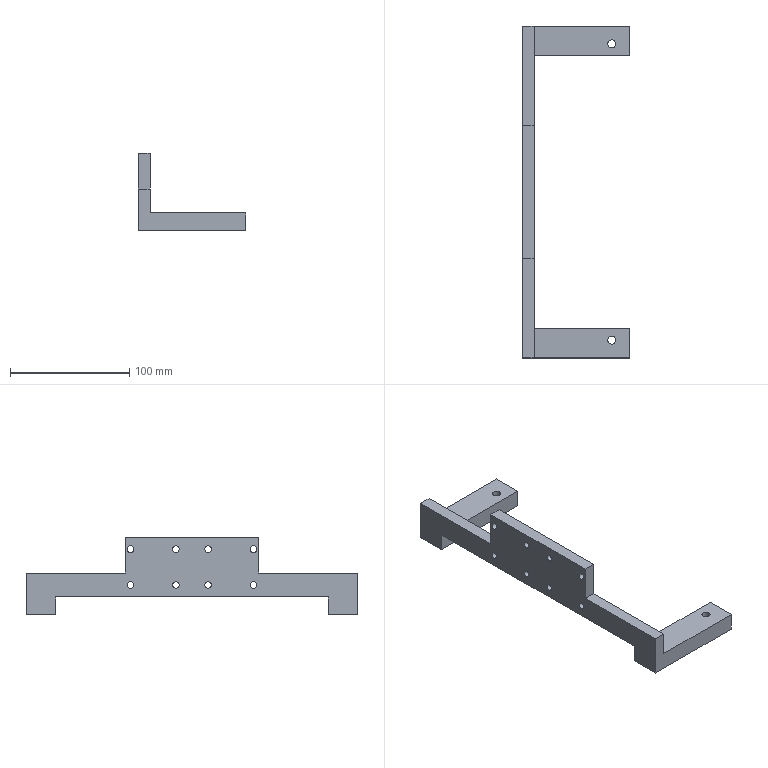Part | 1 solid | 38 faces | box 90 x 278 x 65 mm | volume 153710 mm3 | cylinder 20 | plane 18 | commonest cylinder face diameters 5.5 x16 6.8 x4
STEP:
#1=CARTESIAN_POINT('',(10.,148.5,17.25));
#2=VERTEX_POINT('',#1);
#3=CARTESIAN_POINT('',(10.,148.5,22.75));
#4=VERTEX_POINT('',#3);
#5=CARTESIAN_POINT('',(10.,148.5,20.));
#6=DIRECTION('',(-1.,0.,0.));
#7=DIRECTION('',(0.,0.,1.));
#8=AXIS2_PLACEMENT_3D('',#5,#6,#7);
#9=CIRCLE('',#8,2.75);
#10=EDGE_CURVE('',#2,#4,#9,.T.);
#11=ORIENTED_EDGE('',*,*,#10,.F.);
#12=CARTESIAN_POINT('',(0.,148.5,17.25));
#13=VERTEX_POINT('',#12);
#14=CARTESIAN_POINT('',(10.,148.5,17.25));
#15=DIRECTION('',(-1.,0.,0.));
#16=VECTOR('',#15,1000.);
#17=LINE('',#14,#16);
#18=EDGE_CURVE('',#2,#13,#17,.T.);
#19=ORIENTED_EDGE('',*,*,#18,.T.);
#20=CARTESIAN_POINT('',(0.,148.5,22.75));
#21=VERTEX_POINT('',#20);
#22=CARTESIAN_POINT('',(0.,148.5,20.));
#23=DIRECTION('',(-1.,0.,0.));
#24=DIRECTION('',(0.,0.,1.));
#25=AXIS2_PLACEMENT_3D('',#22,#23,#24);
#26=CIRCLE('',#25,2.75);
#27=EDGE_CURVE('',#13,#21,#26,.T.);
#28=ORIENTED_EDGE('',*,*,#27,.T.);
#29=CARTESIAN_POINT('',(10.,148.5,22.75));
#30=DIRECTION('',(-1.,0.,0.));
#31=VECTOR('',#30,1000.);
#32=LINE('',#29,#31);
#33=EDGE_CURVE('',#4,#21,#32,.T.);
#34=ORIENTED_EDGE('',*,*,#33,.F.);
#35=EDGE_LOOP('',(#11,#19,#28,#34));
#36=FACE_OUTER_BOUND('',#35,.T.);
#37=CARTESIAN_POINT('',(10.,148.5,20.));
#38=DIRECTION('',(-1.,0.,0.));
#39=DIRECTION('',(0.,0.,1.));
#40=AXIS2_PLACEMENT_3D('',#37,#38,#39);
#41=CYLINDRICAL_SURFACE('',#40,2.75);
#42=ADVANCED_FACE('',(#36),#41,.F.);
#43=CARTESIAN_POINT('',(10.,186.5,17.25));
#44=VERTEX_POINT('',#43);
#45=CARTESIAN_POINT('',(10.,186.5,22.75));
#46=VERTEX_POINT('',#45);
#47=CARTESIAN_POINT('',(10.,186.5,20.));
#48=DIRECTION('',(-1.,0.,0.));
#49=DIRECTION('',(0.,0.,1.));
#50=AXIS2_PLACEMENT_3D('',#47,#48,#49);
#51=CIRCLE('',#50,2.75);
#52=EDGE_CURVE('',#44,#46,#51,.T.);
#53=ORIENTED_EDGE('',*,*,#52,.F.);
#54=CARTESIAN_POINT('',(0.,186.5,17.25));
#55=VERTEX_POINT('',#54);
#56=CARTESIAN_POINT('',(10.,186.5,17.25));
#57=DIRECTION('',(-1.,0.,0.));
#58=VECTOR('',#57,1000.);
#59=LINE('',#56,#58);
#60=EDGE_CURVE('',#44,#55,#59,.T.);
#61=ORIENTED_EDGE('',*,*,#60,.T.);
#62=CARTESIAN_POINT('',(0.,186.5,22.75));
#63=VERTEX_POINT('',#62);
#64=CARTESIAN_POINT('',(0.,186.5,20.));
#65=DIRECTION('',(-1.,0.,0.));
#66=DIRECTION('',(0.,0.,1.));
#67=AXIS2_PLACEMENT_3D('',#64,#65,#66);
#68=CIRCLE('',#67,2.75);
#69=EDGE_CURVE('',#55,#63,#68,.T.);
#70=ORIENTED_EDGE('',*,*,#69,.T.);
#71=CARTESIAN_POINT('',(10.,186.5,22.75));
#72=DIRECTION('',(-1.,0.,0.));
#73=VECTOR('',#72,1000.);
#74=LINE('',#71,#73);
#75=EDGE_CURVE('',#46,#63,#74,.T.);
#76=ORIENTED_EDGE('',*,*,#75,.F.);
#77=EDGE_LOOP('',(#53,#61,#70,#76));
#78=FACE_OUTER_BOUND('',#77,.T.);
#79=CARTESIAN_POINT('',(10.,186.5,20.));
#80=DIRECTION('',(-1.,0.,0.));
#81=DIRECTION('',(0.,0.,1.));
#82=AXIS2_PLACEMENT_3D('',#79,#80,#81);
#83=CYLINDRICAL_SURFACE('',#82,2.75);
#84=ADVANCED_FACE('',(#78),#83,.F.);
#85=CARTESIAN_POINT('',(10.,148.5,47.25));
#86=VERTEX_POINT('',#85);
#87=CARTESIAN_POINT('',(10.,148.5,52.75));
#88=VERTEX_POINT('',#87);
#89=CARTESIAN_POINT('',(10.,148.5,50.));
#90=DIRECTION('',(-1.,0.,0.));
#91=DIRECTION('',(0.,0.,1.));
#92=AXIS2_PLACEMENT_3D('',#89,#90,#91);
#93=CIRCLE('',#92,2.75);
#94=EDGE_CURVE('',#86,#88,#93,.T.);
#95=ORIENTED_EDGE('',*,*,#94,.F.);
#96=CARTESIAN_POINT('',(0.,148.5,47.25));
#97=VERTEX_POINT('',#96);
#98=CARTESIAN_POINT('',(10.,148.5,47.25));
#99=DIRECTION('',(-1.,0.,0.));
#100=VECTOR('',#99,1000.);
#101=LINE('',#98,#100);
#102=EDGE_CURVE('',#86,#97,#101,.T.);
#103=ORIENTED_EDGE('',*,*,#102,.T.);
#104=CARTESIAN_POINT('',(0.,148.5,52.75));
#105=VERTEX_POINT('',#104);
#106=CARTESIAN_POINT('',(0.,148.5,50.));
#107=DIRECTION('',(-1.,0.,0.));
#108=DIRECTION('',(0.,0.,1.));
#109=AXIS2_PLACEMENT_3D('',#106,#107,#108);
#110=CIRCLE('',#109,2.75);
#111=EDGE_CURVE('',#97,#105,#110,.T.);
#112=ORIENTED_EDGE('',*,*,#111,.T.);
#113=CARTESIAN_POINT('',(10.,148.5,52.75));
#114=DIRECTION('',(-1.,0.,0.));
#115=VECTOR('',#114,1000.);
#116=LINE('',#113,#115);
#117=EDGE_CURVE('',#88,#105,#116,.T.);
#118=ORIENTED_EDGE('',*,*,#117,.F.);
#119=EDGE_LOOP('',(#95,#103,#112,#118));
#120=FACE_OUTER_BOUND('',#119,.T.);
#121=CARTESIAN_POINT('',(10.,148.5,50.));
#122=DIRECTION('',(-1.,0.,0.));
#123=DIRECTION('',(0.,0.,1.));
#124=AXIS2_PLACEMENT_3D('',#121,#122,#123);
#125=CYLINDRICAL_SURFACE('',#124,2.75);
#126=ADVANCED_FACE('',(#120),#125,.F.);
#127=CARTESIAN_POINT('',(10.,186.5,47.25));
#128=VERTEX_POINT('',#127);
#129=CARTESIAN_POINT('',(10.,186.5,52.75));
#130=VERTEX_POINT('',#129);
#131=CARTESIAN_POINT('',(10.,186.5,50.));
#132=DIRECTION('',(-1.,0.,0.));
#133=DIRECTION('',(0.,0.,1.));
#134=AXIS2_PLACEMENT_3D('',#131,#132,#133);
#135=CIRCLE('',#134,2.75);
#136=EDGE_CURVE('',#128,#130,#135,.T.);
#137=ORIENTED_EDGE('',*,*,#136,.F.);
#138=CARTESIAN_POINT('',(0.,186.5,47.25));
#139=VERTEX_POINT('',#138);
#140=CARTESIAN_POINT('',(10.,186.5,47.25));
#141=DIRECTION('',(-1.,0.,0.));
#142=VECTOR('',#141,1000.);
#143=LINE('',#140,#142);
#144=EDGE_CURVE('',#128,#139,#143,.T.);
#145=ORIENTED_EDGE('',*,*,#144,.T.);
#146=CARTESIAN_POINT('',(0.,186.5,52.75));
#147=VERTEX_POINT('',#146);
#148=CARTESIAN_POINT('',(0.,186.5,50.));
#149=DIRECTION('',(-1.,0.,0.));
#150=DIRECTION('',(0.,0.,1.));
#151=AXIS2_PLACEMENT_3D('',#148,#149,#150);
#152=CIRCLE('',#151,2.75);
#153=EDGE_CURVE('',#139,#147,#152,.T.);
#154=ORIENTED_EDGE('',*,*,#153,.T.);
#155=CARTESIAN_POINT('',(10.,186.5,52.75));
#156=DIRECTION('',(-1.,0.,0.));
#157=VECTOR('',#156,1000.);
#158=LINE('',#155,#157);
#159=EDGE_CURVE('',#130,#147,#158,.T.);
#160=ORIENTED_EDGE('',*,*,#159,.F.);
#161=EDGE_LOOP('',(#137,#145,#154,#160));
#162=FACE_OUTER_BOUND('',#161,.T.);
#163=CARTESIAN_POINT('',(10.,186.5,50.));
#164=DIRECTION('',(-1.,0.,0.));
#165=DIRECTION('',(0.,0.,1.));
#166=AXIS2_PLACEMENT_3D('',#163,#164,#165);
#167=CYLINDRICAL_SURFACE('',#166,2.75);
#168=ADVANCED_FACE('',(#162),#167,.F.);
#169=CARTESIAN_POINT('',(10.,121.5,47.25));
#170=VERTEX_POINT('',#169);
#171=CARTESIAN_POINT('',(10.,121.5,52.75));
#172=VERTEX_POINT('',#171);
#173=CARTESIAN_POINT('',(10.,121.5,50.));
#174=DIRECTION('',(-1.,0.,0.));
#175=DIRECTION('',(0.,0.,1.));
#176=AXIS2_PLACEMENT_3D('',#173,#174,#175);
#177=CIRCLE('',#176,2.75);
#178=EDGE_CURVE('',#170,#172,#177,.T.);
#179=ORIENTED_EDGE('',*,*,#178,.F.);
#180=CARTESIAN_POINT('',(0.,121.5,47.25));
#181=VERTEX_POINT('',#180);
#182=CARTESIAN_POINT('',(10.,121.5,47.25));
#183=DIRECTION('',(-1.,0.,0.));
#184=VECTOR('',#183,1000.);
#185=LINE('',#182,#184);
#186=EDGE_CURVE('',#170,#181,#185,.T.);
#187=ORIENTED_EDGE('',*,*,#186,.T.);
#188=CARTESIAN_POINT('',(0.,121.5,52.75));
#189=VERTEX_POINT('',#188);
#190=CARTESIAN_POINT('',(0.,121.5,50.));
#191=DIRECTION('',(-1.,0.,0.));
#192=DIRECTION('',(0.,0.,1.));
#193=AXIS2_PLACEMENT_3D('',#190,#191,#192);
#194=CIRCLE('',#193,2.75);
#195=EDGE_CURVE('',#181,#189,#194,.T.);
#196=ORIENTED_EDGE('',*,*,#195,.T.);
#197=CARTESIAN_POINT('',(10.,121.5,52.75));
#198=DIRECTION('',(-1.,0.,0.));
#199=VECTOR('',#198,1000.);
#200=LINE('',#197,#199);
#201=EDGE_CURVE('',#172,#189,#200,.T.);
#202=ORIENTED_EDGE('',*,*,#201,.F.);
#203=EDGE_LOOP('',(#179,#187,#196,#202));
#204=FACE_OUTER_BOUND('',#203,.T.);
#205=CARTESIAN_POINT('',(10.,121.5,50.));
#206=DIRECTION('',(-1.,0.,0.));
#207=DIRECTION('',(0.,0.,1.));
#208=AXIS2_PLACEMENT_3D('',#205,#206,#207);
#209=CYLINDRICAL_SURFACE('',#208,2.75);
#210=ADVANCED_FACE('',(#204),#209,.F.);
#211=CARTESIAN_POINT('',(10.,121.5,17.25));
#212=VERTEX_POINT('',#211);
#213=CARTESIAN_POINT('',(10.,121.5,22.75));
#214=VERTEX_POINT('',#213);
#215=CARTESIAN_POINT('',(10.,121.5,20.));
#216=DIRECTION('',(-1.,0.,0.));
#217=DIRECTION('',(0.,0.,1.));
#218=AXIS2_PLACEMENT_3D('',#215,#216,#217);
#219=CIRCLE('',#218,2.75);
#220=EDGE_CURVE('',#212,#214,#219,.T.);
#221=ORIENTED_EDGE('',*,*,#220,.F.);
#222=CARTESIAN_POINT('',(0.,121.5,17.25));
#223=VERTEX_POINT('',#222);
#224=CARTESIAN_POINT('',(10.,121.5,17.25));
#225=DIRECTION('',(-1.,0.,0.));
#226=VECTOR('',#225,1000.);
#227=LINE('',#224,#226);
#228=EDGE_CURVE('',#212,#223,#227,.T.);
#229=ORIENTED_EDGE('',*,*,#228,.T.);
#230=CARTESIAN_POINT('',(0.,121.5,22.75));
#231=VERTEX_POINT('',#230);
#232=CARTESIAN_POINT('',(0.,121.5,20.));
#233=DIRECTION('',(-1.,0.,0.));
#234=DIRECTION('',(0.,0.,1.));
#235=AXIS2_PLACEMENT_3D('',#232,#233,#234);
#236=CIRCLE('',#235,2.75);
#237=EDGE_CURVE('',#223,#231,#236,.T.);
#238=ORIENTED_EDGE('',*,*,#237,.T.);
#239=CARTESIAN_POINT('',(10.,121.5,22.75));
#240=DIRECTION('',(-1.,0.,0.));
#241=VECTOR('',#240,1000.);
#242=LINE('',#239,#241);
#243=EDGE_CURVE('',#214,#231,#242,.T.);
#244=ORIENTED_EDGE('',*,*,#243,.F.);
#245=EDGE_LOOP('',(#221,#229,#238,#244));
#246=FACE_OUTER_BOUND('',#245,.T.);
#247=CARTESIAN_POINT('',(10.,121.5,20.));
#248=DIRECTION('',(-1.,0.,0.));
#249=DIRECTION('',(0.,0.,1.));
#250=AXIS2_PLACEMENT_3D('',#247,#248,#249);
#251=CYLINDRICAL_SURFACE('',#250,2.75);
#252=ADVANCED_FACE('',(#246),#251,.F.);
#253=CARTESIAN_POINT('',(10.,83.5,47.25));
#254=VERTEX_POINT('',#253);
#255=CARTESIAN_POINT('',(10.,83.5,52.75));
#256=VERTEX_POINT('',#255);
#257=CARTESIAN_POINT('',(10.,83.5,50.));
#258=DIRECTION('',(-1.,0.,0.));
#259=DIRECTION('',(0.,0.,1.));
#260=AXIS2_PLACEMENT_3D('',#257,#258,#259);
#261=CIRCLE('',#260,2.75);
#262=EDGE_CURVE('',#254,#256,#261,.T.);
#263=ORIENTED_EDGE('',*,*,#262,.F.);
#264=CARTESIAN_POINT('',(0.,83.5,47.25));
#265=VERTEX_POINT('',#264);
#266=CARTESIAN_POINT('',(10.,83.5,47.25));
#267=DIRECTION('',(-1.,0.,0.));
#268=VECTOR('',#267,1000.);
#269=LINE('',#266,#268);
#270=EDGE_CURVE('',#254,#265,#269,.T.);
#271=ORIENTED_EDGE('',*,*,#270,.T.);
#272=CARTESIAN_POINT('',(0.,83.5,52.75));
#273=VERTEX_POINT('',#272);
#274=CARTESIAN_POINT('',(0.,83.5,50.));
#275=DIRECTION('',(-1.,0.,0.));
#276=DIRECTION('',(0.,0.,1.));
#277=AXIS2_PLACEMENT_3D('',#274,#275,#276);
#278=CIRCLE('',#277,2.75);
#279=EDGE_CURVE('',#265,#273,#278,.T.);
#280=ORIENTED_EDGE('',*,*,#279,.T.);
#281=CARTESIAN_POINT('',(10.,83.5,52.75));
#282=DIRECTION('',(-1.,0.,0.));
#283=VECTOR('',#282,1000.);
#284=LINE('',#281,#283);
#285=EDGE_CURVE('',#256,#273,#284,.T.);
#286=ORIENTED_EDGE('',*,*,#285,.F.);
#287=EDGE_LOOP('',(#263,#271,#280,#286));
#288=FACE_OUTER_BOUND('',#287,.T.);
#289=CARTESIAN_POINT('',(10.,83.5,50.));
#290=DIRECTION('',(-1.,0.,0.));
#291=DIRECTION('',(0.,0.,1.));
#292=AXIS2_PLACEMENT_3D('',#289,#290,#291);
#293=CYLINDRICAL_SURFACE('',#292,2.75);
#294=ADVANCED_FACE('',(#288),#293,.F.);
#295=CARTESIAN_POINT('',(10.,83.5,17.25));
#296=VERTEX_POINT('',#295);
#297=CARTESIAN_POINT('',(10.,83.5,22.75));
#298=VERTEX_POINT('',#297);
#299=CARTESIAN_POINT('',(10.,83.5,20.));
#300=DIRECTION('',(-1.,0.,0.));
#301=DIRECTION('',(0.,0.,1.));
#302=AXIS2_PLACEMENT_3D('',#299,#300,#301);
#303=CIRCLE('',#302,2.75);
#304=EDGE_CURVE('',#296,#298,#303,.T.);
#305=ORIENTED_EDGE('',*,*,#304,.F.);
#306=CARTESIAN_POINT('',(0.,83.5,17.25));
#307=VERTEX_POINT('',#306);
#308=CARTESIAN_POINT('',(10.,83.5,17.25));
#309=DIRECTION('',(-1.,0.,0.));
#310=VECTOR('',#309,1000.);
#311=LINE('',#308,#310);
#312=EDGE_CURVE('',#296,#307,#311,.T.);
#313=ORIENTED_EDGE('',*,*,#312,.T.);
#314=CARTESIAN_POINT('',(0.,83.5,22.75));
#315=VERTEX_POINT('',#314);
#316=CARTESIAN_POINT('',(0.,83.5,20.));
#317=DIRECTION('',(-1.,0.,0.));
#318=DIRECTION('',(0.,0.,1.));
#319=AXIS2_PLACEMENT_3D('',#316,#317,#318);
#320=CIRCLE('',#319,2.75);
#321=EDGE_CURVE('',#307,#315,#320,.T.);
#322=ORIENTED_EDGE('',*,*,#321,.T.);
#323=CARTESIAN_POINT('',(10.,83.5,22.75));
#324=DIRECTION('',(-1.,0.,0.));
#325=VECTOR('',#324,1000.);
#326=LINE('',#323,#325);
#327=EDGE_CURVE('',#298,#315,#326,.T.);
#328=ORIENTED_EDGE('',*,*,#327,.F.);
#329=EDGE_LOOP('',(#305,#313,#322,#328));
#330=FACE_OUTER_BOUND('',#329,.T.);
#331=CARTESIAN_POINT('',(10.,83.5,20.));
#332=DIRECTION('',(-1.,0.,0.));
#333=DIRECTION('',(0.,0.,1.));
#334=AXIS2_PLACEMENT_3D('',#331,#332,#333);
#335=CYLINDRICAL_SURFACE('',#334,2.75);
#336=ADVANCED_FACE('',(#330),#335,.F.);
#337=CARTESIAN_POINT('',(78.4,258.99,-5.));
#338=VERTEX_POINT('',#337);
#339=CARTESIAN_POINT('',(71.6,258.99,-5.));
#340=VERTEX_POINT('',#339);
#341=CARTESIAN_POINT('',(75.,258.99,-5.));
#342=DIRECTION('',(0.,0.,-1.));
#343=DIRECTION('',(-1.,0.,0.));
#344=AXIS2_PLACEMENT_3D('',#341,#342,#343);
#345=CIRCLE('',#344,3.4);
#346=EDGE_CURVE('',#338,#340,#345,.T.);
#347=ORIENTED_EDGE('',*,*,#346,.T.);
#348=CARTESIAN_POINT('',(71.6,258.99,10.));
#349=VERTEX_POINT('',#348);
#350=CARTESIAN_POINT('',(71.6,258.99,10.));
#351=DIRECTION('',(0.,0.,1.));
#352=VECTOR('',#351,1000.);
#353=LINE('',#350,#352);
#354=EDGE_CURVE('',#340,#349,#353,.T.);
#355=ORIENTED_EDGE('',*,*,#354,.T.);
#356=CARTESIAN_POINT('',(78.4,258.99,10.));
#357=VERTEX_POINT('',#356);
#358=CARTESIAN_POINT('',(75.,258.99,10.));
#359=DIRECTION('',(0.,0.,1.));
#360=DIRECTION('',(1.,0.,0.));
#361=AXIS2_PLACEMENT_3D('',#358,#359,#360);
#362=CIRCLE('',#361,3.4);
#363=EDGE_CURVE('',#349,#357,#362,.T.);
#364=ORIENTED_EDGE('',*,*,#363,.T.);
#365=CARTESIAN_POINT('',(78.4,258.99,10.));
#366=DIRECTION('',(0.,0.,1.));
#367=VECTOR('',#366,1000.);
#368=LINE('',#365,#367);
#369=EDGE_CURVE('',#338,#357,#368,.T.);
#370=ORIENTED_EDGE('',*,*,#369,.F.);
#371=EDGE_LOOP('',(#347,#355,#364,#370));
#372=FACE_OUTER_BOUND('',#371,.T.);
#373=CARTESIAN_POINT('',(75.,258.99,10.));
#374=DIRECTION('',(0.,0.,1.));
#375=DIRECTION('',(1.,0.,0.));
#376=AXIS2_PLACEMENT_3D('',#373,#374,#375);
#377=CYLINDRICAL_SURFACE('',#376,3.4);
#378=ADVANCED_FACE('',(#372),#377,.F.);
#379=CARTESIAN_POINT('',(78.4,11.01,-5.));
#380=VERTEX_POINT('',#379);
#381=CARTESIAN_POINT('',(71.6,11.01,-5.));
#382=VERTEX_POINT('',#381);
#383=CARTESIAN_POINT('',(75.,11.01,-5.));
#384=DIRECTION('',(0.,0.,-1.));
#385=DIRECTION('',(-1.,0.,0.));
#386=AXIS2_PLACEMENT_3D('',#383,#384,#385);
#387=CIRCLE('',#386,3.4);
#388=EDGE_CURVE('',#380,#382,#387,.T.);
#389=ORIENTED_EDGE('',*,*,#388,.T.);
#390=CARTESIAN_POINT('',(71.6,11.01,10.));
#391=VERTEX_POINT('',#390);
#392=CARTESIAN_POINT('',(71.6,11.01,10.));
#393=DIRECTION('',(0.,0.,1.));
#394=VECTOR('',#393,1000.);
#395=LINE('',#392,#394);
#396=EDGE_CURVE('',#382,#391,#395,.T.);
#397=ORIENTED_EDGE('',*,*,#396,.T.);
#398=CARTESIAN_POINT('',(78.4,11.01,10.));
#399=VERTEX_POINT('',#398);
#400=CARTESIAN_POINT('',(75.,11.01,10.));
#401=DIRECTION('',(0.,0.,1.));
#402=DIRECTION('',(1.,0.,0.));
#403=AXIS2_PLACEMENT_3D('',#400,#401,#402);
#404=CIRCLE('',#403,3.4);
#405=EDGE_CURVE('',#391,#399,#404,.T.);
#406=ORIENTED_EDGE('',*,*,#405,.T.);
#407=CARTESIAN_POINT('',(78.4,11.01,10.));
#408=DIRECTION('',(0.,0.,1.));
#409=VECTOR('',#408,1000.);
#410=LINE('',#407,#409);
#411=EDGE_CURVE('',#380,#399,#410,.T.);
#412=ORIENTED_EDGE('',*,*,#411,.F.);
#413=EDGE_LOOP('',(#389,#397,#406,#412));
#414=FACE_OUTER_BOUND('',#413,.T.);
#415=CARTESIAN_POINT('',(75.,11.01,10.));
#416=DIRECTION('',(0.,0.,1.));
#417=DIRECTION('',(1.,0.,0.));
#418=AXIS2_PLACEMENT_3D('',#415,#416,#417);
#419=CYLINDRICAL_SURFACE('',#418,3.4);
#420=ADVANCED_FACE('',(#414),#419,.F.);
#421=ORIENTED_EDGE('',*,*,#388,.F.);
#422=CARTESIAN_POINT('',(75.,11.01,-5.));
#423=DIRECTION('',(0.,0.,-1.));
#424=DIRECTION('',(-1.,0.,0.));
#425=AXIS2_PLACEMENT_3D('',#422,#423,#424);
#426=CIRCLE('',#425,3.4);
#427=EDGE_CURVE('',#382,#380,#426,.T.);
#428=ORIENTED_EDGE('',*,*,#427,.F.);
#429=EDGE_LOOP('',(#421,#428));
#430=FACE_BOUND('',#429,.T.);
#431=CARTESIAN_POINT('',(0.,-4.,-5.));
#432=VERTEX_POINT('',#431);
#433=CARTESIAN_POINT('',(0.,21.,-5.));
#434=VERTEX_POINT('',#433);
#435=CARTESIAN_POINT('',(0.,41.,-5.));
#436=DIRECTION('',(0.,1.,0.));
#437=VECTOR('',#436,1000.);
#438=LINE('',#435,#437);
#439=EDGE_CURVE('',#432,#434,#438,.T.);
#440=ORIENTED_EDGE('',*,*,#439,.T.);
#441=CARTESIAN_POINT('',(90.,21.,-5.));
#442=VERTEX_POINT('',#441);
#443=CARTESIAN_POINT('',(0.,21.,-5.));
#444=DIRECTION('',(-1.,0.,0.));
#445=VECTOR('',#444,1000.);
#446=LINE('',#443,#445);
#447=EDGE_CURVE('',#442,#434,#446,.T.);
#448=ORIENTED_EDGE('',*,*,#447,.F.);
#449=CARTESIAN_POINT('',(90.,-4.,-5.));
#450=VERTEX_POINT('',#449);
#451=CARTESIAN_POINT('',(90.,41.,-5.));
#452=DIRECTION('',(0.,-1.,0.));
#453=VECTOR('',#452,1000.);
#454=LINE('',#451,#453);
#455=EDGE_CURVE('',#442,#450,#454,.T.);
#456=ORIENTED_EDGE('',*,*,#455,.T.);
#457=CARTESIAN_POINT('',(90.,-4.,-5.));
#458=DIRECTION('',(-1.,0.,0.));
#459=VECTOR('',#458,1000.);
#460=LINE('',#457,#459);
#461=EDGE_CURVE('',#450,#432,#460,.T.);
#462=ORIENTED_EDGE('',*,*,#461,.T.);
#463=EDGE_LOOP('',(#440,#448,#456,#462));
#464=FACE_OUTER_BOUND('',#463,.T.);
#465=CARTESIAN_POINT('',(0.,0.,-5.));
#466=DIRECTION('',(0.,0.,-1.));
#467=DIRECTION('',(-1.,0.,0.));
#468=AXIS2_PLACEMENT_3D('',#465,#466,#467);
#469=PLANE('',#468);
#470=ADVANCED_FACE('',(#430,#464),#469,.T.);
#471=ORIENTED_EDGE('',*,*,#346,.F.);
#472=CARTESIAN_POINT('',(75.,258.99,-5.));
#473=DIRECTION('',(0.,0.,-1.));
#474=DIRECTION('',(-1.,0.,0.));
#475=AXIS2_PLACEMENT_3D('',#472,#473,#474);
#476=CIRCLE('',#475,3.4);
#477=EDGE_CURVE('',#340,#338,#476,.T.);
#478=ORIENTED_EDGE('',*,*,#477,.F.);
#479=EDGE_LOOP('',(#471,#478));
#480=FACE_BOUND('',#479,.T.);
#481=CARTESIAN_POINT('',(0.,249.,-5.));
#482=VERTEX_POINT('',#481);
#483=CARTESIAN_POINT('',(90.,249.,-5.));
#484=VERTEX_POINT('',#483);
#485=CARTESIAN_POINT('',(0.,249.,-5.));
#486=DIRECTION('',(1.,0.,0.));
#487=VECTOR('',#486,1000.);
#488=LINE('',#485,#487);
#489=EDGE_CURVE('',#482,#484,#488,.T.);
#490=ORIENTED_EDGE('',*,*,#489,.F.);
#491=CARTESIAN_POINT('',(0.,274.,-5.));
#492=VERTEX_POINT('',#491);
#493=CARTESIAN_POINT('',(0.,254.,-5.));
#494=DIRECTION('',(0.,1.,0.));
#495=VECTOR('',#494,1000.);
#496=LINE('',#493,#495);
#497=EDGE_CURVE('',#482,#492,#496,.T.);
#498=ORIENTED_EDGE('',*,*,#497,.T.);
#499=CARTESIAN_POINT('',(90.,274.,-5.));
#500=VERTEX_POINT('',#499);
#501=CARTESIAN_POINT('',(90.,274.,-5.));
#502=DIRECTION('',(-1.,0.,0.));
#503=VECTOR('',#502,1000.);
#504=LINE('',#501,#503);
#505=EDGE_CURVE('',#500,#492,#504,.T.);
#506=ORIENTED_EDGE('',*,*,#505,.F.);
#507=CARTESIAN_POINT('',(90.,254.,-5.));
#508=DIRECTION('',(0.,-1.,0.));
#509=VECTOR('',#508,1000.);
#510=LINE('',#507,#509);
#511=EDGE_CURVE('',#500,#484,#510,.T.);
#512=ORIENTED_EDGE('',*,*,#511,.T.);
#513=EDGE_LOOP('',(#490,#498,#506,#512));
#514=FACE_OUTER_BOUND('',#513,.T.);
#515=CARTESIAN_POINT('',(0.,0.,-5.));
#516=DIRECTION('',(0.,0.,-1.));
#517=DIRECTION('',(-1.,0.,0.));
#518=AXIS2_PLACEMENT_3D('',#515,#516,#517);
#519=PLANE('',#518);
#520=ADVANCED_FACE('',(#480,#514),#519,.T.);
#521=CARTESIAN_POINT('',(10.,21.,10.));
#522=VERTEX_POINT('',#521);
#523=CARTESIAN_POINT('',(10.,249.,10.));
#524=VERTEX_POINT('',#523);
#525=CARTESIAN_POINT('',(10.,41.,10.));
#526=DIRECTION('',(0.,1.,0.));
#527=VECTOR('',#526,1000.);
#528=LINE('',#525,#527);
#529=EDGE_CURVE('',#522,#524,#528,.T.);
#530=ORIENTED_EDGE('',*,*,#529,.F.);
#531=CARTESIAN_POINT('',(0.,21.,10.));
#532=VERTEX_POINT('',#531);
#533=CARTESIAN_POINT('',(0.,21.,10.));
#534=DIRECTION('',(1.,0.,0.));
#535=VECTOR('',#534,1000.);
#536=LINE('',#533,#535);
#537=EDGE_CURVE('',#532,#522,#536,.T.);
#538=ORIENTED_EDGE('',*,*,#537,.F.);
#539=CARTESIAN_POINT('',(0.,249.,10.));
#540=VERTEX_POINT('',#539);
#541=CARTESIAN_POINT('',(0.,-120.,10.));
#542=DIRECTION('',(0.,1.,0.));
#543=VECTOR('',#542,1000.);
#544=LINE('',#541,#543);
#545=EDGE_CURVE('',#532,#540,#544,.T.);
#546=ORIENTED_EDGE('',*,*,#545,.T.);
#547=CARTESIAN_POINT('',(10.,249.,10.));
#548=DIRECTION('',(-1.,0.,0.));
#549=VECTOR('',#548,1000.);
#550=LINE('',#547,#549);
#551=EDGE_CURVE('',#524,#540,#550,.T.);
#552=ORIENTED_EDGE('',*,*,#551,.F.);
#553=EDGE_LOOP('',(#530,#538,#546,#552));
#554=FACE_OUTER_BOUND('',#553,.T.);
#555=CARTESIAN_POINT('',(0.,-120.,10.));
#556=DIRECTION('',(0.,0.,1.));
#557=DIRECTION('',(1.,0.,0.));
#558=AXIS2_PLACEMENT_3D('',#555,#556,#557);
#559=PLANE('',#558);
#560=ADVANCED_FACE('',(#554),#559,.F.);
#561=CARTESIAN_POINT('',(90.,249.,10.));
#562=VERTEX_POINT('',#561);
#563=CARTESIAN_POINT('',(90.,274.,10.));
#564=VERTEX_POINT('',#563);
#565=CARTESIAN_POINT('',(90.,-12.,10.));
#566=DIRECTION('',(0.,1.,0.));
#567=VECTOR('',#566,1000.);
#568=LINE('',#565,#567);
#569=EDGE_CURVE('',#562,#564,#568,.T.);
#570=ORIENTED_EDGE('',*,*,#569,.F.);
#571=CARTESIAN_POINT('',(90.,249.,-10.));
#572=DIRECTION('',(0.,0.,1.));
#573=VECTOR('',#572,1000.);
#574=LINE('',#571,#573);
#575=EDGE_CURVE('',#484,#562,#574,.T.);
#576=ORIENTED_EDGE('',*,*,#575,.F.);
#577=ORIENTED_EDGE('',*,*,#511,.F.);
#578=CARTESIAN_POINT('',(90.,274.,10.));
#579=DIRECTION('',(0.,0.,-1.));
#580=VECTOR('',#579,1000.);
#581=LINE('',#578,#580);
#582=EDGE_CURVE('',#564,#500,#581,.T.);
#583=ORIENTED_EDGE('',*,*,#582,.F.);
#584=EDGE_LOOP('',(#570,#576,#577,#583));
#585=FACE_OUTER_BOUND('',#584,.T.);
#586=CARTESIAN_POINT('',(90.,0.,0.));
#587=DIRECTION('',(-1.,0.,0.));
#588=DIRECTION('',(0.,-1.,0.));
#589=AXIS2_PLACEMENT_3D('',#586,#587,#588);
#590=PLANE('',#589);
#591=ADVANCED_FACE('',(#585),#590,.F.);
#592=CARTESIAN_POINT('',(10.,148.5,20.));
#593=DIRECTION('',(-1.,0.,0.));
#594=DIRECTION('',(0.,0.,1.));
#595=AXIS2_PLACEMENT_3D('',#592,#593,#594);
#596=CIRCLE('',#595,2.75);
#597=EDGE_CURVE('',#4,#2,#596,.T.);
#598=ORIENTED_EDGE('',*,*,#597,.T.);
#599=ORIENTED_EDGE('',*,*,#10,.T.);
#600=EDGE_LOOP('',(#598,#599));
#601=FACE_BOUND('',#600,.T.);
#602=CARTESIAN_POINT('',(10.,186.5,20.));
#603=DIRECTION('',(-1.,0.,0.));
#604=DIRECTION('',(0.,0.,1.));
#605=AXIS2_PLACEMENT_3D('',#602,#603,#604);
#606=CIRCLE('',#605,2.75);
#607=EDGE_CURVE('',#46,#44,#606,.T.);
#608=ORIENTED_EDGE('',*,*,#607,.T.);
#609=ORIENTED_EDGE('',*,*,#52,.T.);
#610=EDGE_LOOP('',(#608,#609));
#611=FACE_BOUND('',#610,.T.);
#612=CARTESIAN_POINT('',(10.,148.5,50.));
#613=DIRECTION('',(-1.,0.,0.));
#614=DIRECTION('',(0.,0.,1.));
#615=AXIS2_PLACEMENT_3D('',#612,#613,#614);
#616=CIRCLE('',#615,2.75);
#617=EDGE_CURVE('',#88,#86,#616,.T.);
#618=ORIENTED_EDGE('',*,*,#617,.T.);
#619=ORIENTED_EDGE('',*,*,#94,.T.);
#620=EDGE_LOOP('',(#618,#619));
#621=FACE_BOUND('',#620,.T.);
#622=CARTESIAN_POINT('',(10.,186.5,50.));
#623=DIRECTION('',(-1.,0.,0.));
#624=DIRECTION('',(0.,0.,1.));
#625=AXIS2_PLACEMENT_3D('',#622,#623,#624);
#626=CIRCLE('',#625,2.75);
#627=EDGE_CURVE('',#130,#128,#626,.T.);
#628=ORIENTED_EDGE('',*,*,#627,.T.);
#629=ORIENTED_EDGE('',*,*,#136,.T.);
#630=EDGE_LOOP('',(#628,#629));
#631=FACE_BOUND('',#630,.T.);
#632=CARTESIAN_POINT('',(10.,121.5,50.));
#633=DIRECTION('',(-1.,0.,0.));
#634=DIRECTION('',(0.,0.,1.));
#635=AXIS2_PLACEMENT_3D('',#632,#633,#634);
#636=CIRCLE('',#635,2.75);
#637=EDGE_CURVE('',#172,#170,#636,.T.);
#638=ORIENTED_EDGE('',*,*,#637,.T.);
#639=ORIENTED_EDGE('',*,*,#178,.T.);
#640=EDGE_LOOP('',(#638,#639));
#641=FACE_BOUND('',#640,.T.);
#642=CARTESIAN_POINT('',(10.,121.5,20.));
#643=DIRECTION('',(-1.,0.,0.));
#644=DIRECTION('',(0.,0.,1.));
#645=AXIS2_PLACEMENT_3D('',#642,#643,#644);
#646=CIRCLE('',#645,2.75);
#647=EDGE_CURVE('',#214,#212,#646,.T.);
#648=ORIENTED_EDGE('',*,*,#647,.T.);
#649=ORIENTED_EDGE('',*,*,#220,.T.);
#650=EDGE_LOOP('',(#648,#649));
#651=FACE_BOUND('',#650,.T.);
#652=CARTESIAN_POINT('',(10.,83.5,50.));
#653=DIRECTION('',(-1.,0.,0.));
#654=DIRECTION('',(0.,0.,1.));
#655=AXIS2_PLACEMENT_3D('',#652,#653,#654);
#656=CIRCLE('',#655,2.75);
#657=EDGE_CURVE('',#256,#254,#656,.T.);
#658=ORIENTED_EDGE('',*,*,#657,.T.);
#659=ORIENTED_EDGE('',*,*,#262,.T.);
#660=EDGE_LOOP('',(#658,#659));
#661=FACE_BOUND('',#660,.T.);
#662=CARTESIAN_POINT('',(10.,83.5,20.));
#663=DIRECTION('',(-1.,0.,0.));
#664=DIRECTION('',(0.,0.,1.));
#665=AXIS2_PLACEMENT_3D('',#662,#663,#664);
#666=CIRCLE('',#665,2.75);
#667=EDGE_CURVE('',#298,#296,#666,.T.);
#668=ORIENTED_EDGE('',*,*,#667,.T.);
#669=ORIENTED_EDGE('',*,*,#304,.T.);
#670=EDGE_LOOP('',(#668,#669));
#671=FACE_BOUND('',#670,.T.);
#672=CARTESIAN_POINT('',(10.,-4.,10.));
#673=VERTEX_POINT('',#672);
#674=CARTESIAN_POINT('',(10.,-12.,10.));
#675=DIRECTION('',(0.,1.,0.));
#676=VECTOR('',#675,1000.);
#677=LINE('',#674,#676);
#678=EDGE_CURVE('',#673,#522,#677,.T.);
#679=ORIENTED_EDGE('',*,*,#678,.T.);
#680=ORIENTED_EDGE('',*,*,#529,.T.);
#681=CARTESIAN_POINT('',(10.,274.,10.));
#682=VERTEX_POINT('',#681);
#683=CARTESIAN_POINT('',(10.,-12.,10.));
#684=DIRECTION('',(0.,1.,0.));
#685=VECTOR('',#684,1000.);
#686=LINE('',#683,#685);
#687=EDGE_CURVE('',#524,#682,#686,.T.);
#688=ORIENTED_EDGE('',*,*,#687,.T.);
#689=CARTESIAN_POINT('',(10.,274.,30.));
#690=VERTEX_POINT('',#689);
#691=CARTESIAN_POINT('',(10.,274.,30.));
#692=DIRECTION('',(0.,0.,-1.));
#693=VECTOR('',#692,1000.);
#694=LINE('',#691,#693);
#695=EDGE_CURVE('',#690,#682,#694,.T.);
#696=ORIENTED_EDGE('',*,*,#695,.F.);
#697=CARTESIAN_POINT('',(10.,191.,30.));
#698=VERTEX_POINT('',#697);
#699=CARTESIAN_POINT('',(10.,254.,30.));
#700=DIRECTION('',(0.,1.,0.));
#701=VECTOR('',#700,1000.);
#702=LINE('',#699,#701);
#703=EDGE_CURVE('',#698,#690,#702,.T.);
#704=ORIENTED_EDGE('',*,*,#703,.F.);
#705=CARTESIAN_POINT('',(10.,191.,60.));
#706=VERTEX_POINT('',#705);
#707=CARTESIAN_POINT('',(10.,191.,60.));
#708=DIRECTION('',(0.,0.,-1.));
#709=VECTOR('',#708,1000.);
#710=LINE('',#707,#709);
#711=EDGE_CURVE('',#706,#698,#710,.T.);
#712=ORIENTED_EDGE('',*,*,#711,.F.);
#713=CARTESIAN_POINT('',(10.,79.,60.));
#714=VERTEX_POINT('',#713);
#715=CARTESIAN_POINT('',(10.,170.,60.));
#716=DIRECTION('',(0.,1.,0.));
#717=VECTOR('',#716,1000.);
#718=LINE('',#715,#717);
#719=EDGE_CURVE('',#714,#706,#718,.T.);
#720=ORIENTED_EDGE('',*,*,#719,.F.);
#721=CARTESIAN_POINT('',(10.,79.,30.));
#722=VERTEX_POINT('',#721);
#723=CARTESIAN_POINT('',(10.,79.,60.));
#724=DIRECTION('',(0.,0.,1.));
#725=VECTOR('',#724,1000.);
#726=LINE('',#723,#725);
#727=EDGE_CURVE('',#722,#714,#726,.T.);
#728=ORIENTED_EDGE('',*,*,#727,.F.);
#729=CARTESIAN_POINT('',(10.,-4.,30.));
#730=VERTEX_POINT('',#729);
#731=CARTESIAN_POINT('',(10.,16.,30.));
#732=DIRECTION('',(0.,1.,0.));
#733=VECTOR('',#732,1000.);
#734=LINE('',#731,#733);
#735=EDGE_CURVE('',#730,#722,#734,.T.);
#736=ORIENTED_EDGE('',*,*,#735,.F.);
#737=CARTESIAN_POINT('',(10.,-4.,30.));
#738=DIRECTION('',(0.,0.,-1.));
#739=VECTOR('',#738,1000.);
#740=LINE('',#737,#739);
#741=EDGE_CURVE('',#730,#673,#740,.T.);
#742=ORIENTED_EDGE('',*,*,#741,.T.);
#743=EDGE_LOOP('',(#679,#680,#688,#696,#704,#712,#720,#728,#736,#742));
#744=FACE_OUTER_BOUND('',#743,.T.);
#745=CARTESIAN_POINT('',(10.,170.,60.));
#746=DIRECTION('',(-1.,0.,0.));
#747=DIRECTION('',(0.,-1.,0.));
#748=AXIS2_PLACEMENT_3D('',#745,#746,#747);
#749=PLANE('',#748);
#750=ADVANCED_FACE('',(#601,#611,#621,#631,#641,#651,#661,#671,#744),#749,.F.);
#751=CARTESIAN_POINT('',(0.,148.5,20.));
#752=DIRECTION('',(-1.,0.,0.));
#753=DIRECTION('',(0.,0.,1.));
#754=AXIS2_PLACEMENT_3D('',#751,#752,#753);
#755=CIRCLE('',#754,2.75);
#756=EDGE_CURVE('',#21,#13,#755,.T.);
#757=ORIENTED_EDGE('',*,*,#756,.F.);
#758=ORIENTED_EDGE('',*,*,#27,.F.);
#759=EDGE_LOOP('',(#757,#758));
#760=FACE_BOUND('',#759,.T.);
#761=CARTESIAN_POINT('',(0.,186.5,20.));
#762=DIRECTION('',(-1.,0.,0.));
#763=DIRECTION('',(0.,0.,1.));
#764=AXIS2_PLACEMENT_3D('',#761,#762,#763);
#765=CIRCLE('',#764,2.75);
#766=EDGE_CURVE('',#63,#55,#765,.T.);
#767=ORIENTED_EDGE('',*,*,#766,.F.);
#768=ORIENTED_EDGE('',*,*,#69,.F.);
#769=EDGE_LOOP('',(#767,#768));
#770=FACE_BOUND('',#769,.T.);
#771=CARTESIAN_POINT('',(0.,148.5,50.));
#772=DIRECTION('',(-1.,0.,0.));
#773=DIRECTION('',(0.,0.,1.));
#774=AXIS2_PLACEMENT_3D('',#771,#772,#773);
#775=CIRCLE('',#774,2.75);
#776=EDGE_CURVE('',#105,#97,#775,.T.);
#777=ORIENTED_EDGE('',*,*,#776,.F.);
#778=ORIENTED_EDGE('',*,*,#111,.F.);
#779=EDGE_LOOP('',(#777,#778));
#780=FACE_BOUND('',#779,.T.);
#781=CARTESIAN_POINT('',(0.,186.5,50.));
#782=DIRECTION('',(-1.,0.,0.));
#783=DIRECTION('',(0.,0.,1.));
#784=AXIS2_PLACEMENT_3D('',#781,#782,#783);
#785=CIRCLE('',#784,2.75);
#786=EDGE_CURVE('',#147,#139,#785,.T.);
#787=ORIENTED_EDGE('',*,*,#786,.F.);
#788=ORIENTED_EDGE('',*,*,#153,.F.);
#789=EDGE_LOOP('',(#787,#788));
#790=FACE_BOUND('',#789,.T.);
#791=CARTESIAN_POINT('',(0.,121.5,50.));
#792=DIRECTION('',(-1.,0.,0.));
#793=DIRECTION('',(0.,0.,1.));
#794=AXIS2_PLACEMENT_3D('',#791,#792,#793);
#795=CIRCLE('',#794,2.75);
#796=EDGE_CURVE('',#189,#181,#795,.T.);
#797=ORIENTED_EDGE('',*,*,#796,.F.);
#798=ORIENTED_EDGE('',*,*,#195,.F.);
#799=EDGE_LOOP('',(#797,#798));
#800=FACE_BOUND('',#799,.T.);
#801=CARTESIAN_POINT('',(0.,121.5,20.));
#802=DIRECTION('',(-1.,0.,0.));
#803=DIRECTION('',(0.,0.,1.));
#804=AXIS2_PLACEMENT_3D('',#801,#802,#803);
#805=CIRCLE('',#804,2.75);
#806=EDGE_CURVE('',#231,#223,#805,.T.);
#807=ORIENTED_EDGE('',*,*,#806,.F.);
#808=ORIENTED_EDGE('',*,*,#237,.F.);
#809=EDGE_LOOP('',(#807,#808));
#810=FACE_BOUND('',#809,.T.);
#811=CARTESIAN_POINT('',(0.,83.5,50.));
#812=DIRECTION('',(-1.,0.,0.));
#813=DIRECTION('',(0.,0.,1.));
#814=AXIS2_PLACEMENT_3D('',#811,#812,#813);
#815=CIRCLE('',#814,2.75);
#816=EDGE_CURVE('',#273,#265,#815,.T.);
#817=ORIENTED_EDGE('',*,*,#816,.F.);
#818=ORIENTED_EDGE('',*,*,#279,.F.);
#819=EDGE_LOOP('',(#817,#818));
#820=FACE_BOUND('',#819,.T.);
#821=CARTESIAN_POINT('',(0.,83.5,20.));
#822=DIRECTION('',(-1.,0.,0.));
#823=DIRECTION('',(0.,0.,1.));
#824=AXIS2_PLACEMENT_3D('',#821,#822,#823);
#825=CIRCLE('',#824,2.75);
#826=EDGE_CURVE('',#315,#307,#825,.T.);
#827=ORIENTED_EDGE('',*,*,#826,.F.);
#828=ORIENTED_EDGE('',*,*,#321,.F.);
#829=EDGE_LOOP('',(#827,#828));
#830=FACE_BOUND('',#829,.T.);
#831=ORIENTED_EDGE('',*,*,#545,.F.);
#832=CARTESIAN_POINT('',(0.,21.,-5.));
#833=DIRECTION('',(0.,0.,1.));
#834=VECTOR('',#833,1000.);
#835=LINE('',#832,#834);
#836=EDGE_CURVE('',#434,#532,#835,.T.);
#837=ORIENTED_EDGE('',*,*,#836,.F.);
#838=ORIENTED_EDGE('',*,*,#439,.F.);
#839=CARTESIAN_POINT('',(0.,-4.,30.));
#840=VERTEX_POINT('',#839);
#841=CARTESIAN_POINT('',(0.,-4.,-5.));
#842=DIRECTION('',(0.,0.,1.));
#843=VECTOR('',#842,1000.);
#844=LINE('',#841,#843);
#845=EDGE_CURVE('',#432,#840,#844,.T.);
#846=ORIENTED_EDGE('',*,*,#845,.T.);
#847=CARTESIAN_POINT('',(0.,79.,30.));
#848=VERTEX_POINT('',#847);
#849=CARTESIAN_POINT('',(0.,0.,30.));
#850=DIRECTION('',(0.,1.,0.));
#851=VECTOR('',#850,1000.);
#852=LINE('',#849,#851);
#853=EDGE_CURVE('',#840,#848,#852,.T.);
#854=ORIENTED_EDGE('',*,*,#853,.T.);
#855=CARTESIAN_POINT('',(0.,79.,60.));
#856=VERTEX_POINT('',#855);
#857=CARTESIAN_POINT('',(0.,79.,10.));
#858=DIRECTION('',(0.,0.,1.));
#859=VECTOR('',#858,1000.);
#860=LINE('',#857,#859);
#861=EDGE_CURVE('',#848,#856,#860,.T.);
#862=ORIENTED_EDGE('',*,*,#861,.T.);
#863=CARTESIAN_POINT('',(0.,191.,60.));
#864=VERTEX_POINT('',#863);
#865=CARTESIAN_POINT('',(0.,170.,60.));
#866=DIRECTION('',(0.,-1.,0.));
#867=VECTOR('',#866,1000.);
#868=LINE('',#865,#867);
#869=EDGE_CURVE('',#864,#856,#868,.T.);
#870=ORIENTED_EDGE('',*,*,#869,.F.);
#871=CARTESIAN_POINT('',(0.,191.,30.));
#872=VERTEX_POINT('',#871);
#873=CARTESIAN_POINT('',(0.,191.,10.));
#874=DIRECTION('',(0.,0.,-1.));
#875=VECTOR('',#874,1000.);
#876=LINE('',#873,#875);
#877=EDGE_CURVE('',#864,#872,#876,.T.);
#878=ORIENTED_EDGE('',*,*,#877,.T.);
#879=CARTESIAN_POINT('',(0.,274.,30.));
#880=VERTEX_POINT('',#879);
#881=CARTESIAN_POINT('',(0.,0.,30.));
#882=DIRECTION('',(0.,1.,0.));
#883=VECTOR('',#882,1000.);
#884=LINE('',#881,#883);
#885=EDGE_CURVE('',#872,#880,#884,.T.);
#886=ORIENTED_EDGE('',*,*,#885,.T.);
#887=CARTESIAN_POINT('',(0.,274.,-5.));
#888=DIRECTION('',(0.,0.,1.));
#889=VECTOR('',#888,1000.);
#890=LINE('',#887,#889);
#891=EDGE_CURVE('',#492,#880,#890,.T.);
#892=ORIENTED_EDGE('',*,*,#891,.F.);
#893=ORIENTED_EDGE('',*,*,#497,.F.);
#894=CARTESIAN_POINT('',(0.,249.,10.));
#895=DIRECTION('',(0.,0.,-1.));
#896=VECTOR('',#895,1000.);
#897=LINE('',#894,#896);
#898=EDGE_CURVE('',#540,#482,#897,.T.);
#899=ORIENTED_EDGE('',*,*,#898,.F.);
#900=EDGE_LOOP('',(#831,#837,#838,#846,#854,#862,#870,#878,#886,#892,#893,#899));
#901=FACE_OUTER_BOUND('',#900,.T.);
#902=CARTESIAN_POINT('',(0.,0.,10.));
#903=DIRECTION('',(1.,0.,0.));
#904=DIRECTION('',(0.,0.,-1.));
#905=AXIS2_PLACEMENT_3D('',#902,#903,#904);
#906=PLANE('',#905);
#907=ADVANCED_FACE('',(#760,#770,#780,#790,#800,#810,#820,#830,#901),#906,.F.);
#908=CARTESIAN_POINT('',(-70.,79.,60.));
#909=DIRECTION('',(1.,0.,0.));
#910=VECTOR('',#909,1000.);
#911=LINE('',#908,#910);
#912=EDGE_CURVE('',#856,#714,#911,.T.);
#913=ORIENTED_EDGE('',*,*,#912,.T.);
#914=ORIENTED_EDGE('',*,*,#719,.T.);
#915=CARTESIAN_POINT('',(-70.,191.,60.));
#916=DIRECTION('',(1.,0.,0.));
#917=VECTOR('',#916,1000.);
#918=LINE('',#915,#917);
#919=EDGE_CURVE('',#864,#706,#918,.T.);
#920=ORIENTED_EDGE('',*,*,#919,.F.);
#921=ORIENTED_EDGE('',*,*,#869,.T.);
#922=EDGE_LOOP('',(#913,#914,#920,#921));
#923=FACE_OUTER_BOUND('',#922,.T.);
#924=CARTESIAN_POINT('',(0.,0.,60.));
#925=DIRECTION('',(0.,0.,1.));
#926=DIRECTION('',(1.,0.,0.));
#927=AXIS2_PLACEMENT_3D('',#924,#925,#926);
#928=PLANE('',#927);
#929=ADVANCED_FACE('',(#923),#928,.T.);
#930=ORIENTED_EDGE('',*,*,#455,.F.);
#931=CARTESIAN_POINT('',(90.,21.,10.));
#932=VERTEX_POINT('',#931);
#933=CARTESIAN_POINT('',(90.,21.,-10.));
#934=DIRECTION('',(0.,0.,1.));
#935=VECTOR('',#934,1000.);
#936=LINE('',#933,#935);
#937=EDGE_CURVE('',#442,#932,#936,.T.);
#938=ORIENTED_EDGE('',*,*,#937,.T.);
#939=CARTESIAN_POINT('',(90.,-4.,10.));
#940=VERTEX_POINT('',#939);
#941=CARTESIAN_POINT('',(90.,-12.,10.));
#942=DIRECTION('',(0.,1.,0.));
#943=VECTOR('',#942,1000.);
#944=LINE('',#941,#943);
#945=EDGE_CURVE('',#940,#932,#944,.T.);
#946=ORIENTED_EDGE('',*,*,#945,.F.);
#947=CARTESIAN_POINT('',(90.,-4.,10.));
#948=DIRECTION('',(0.,0.,-1.));
#949=VECTOR('',#948,1000.);
#950=LINE('',#947,#949);
#951=EDGE_CURVE('',#940,#450,#950,.T.);
#952=ORIENTED_EDGE('',*,*,#951,.T.);
#953=EDGE_LOOP('',(#930,#938,#946,#952));
#954=FACE_OUTER_BOUND('',#953,.T.);
#955=CARTESIAN_POINT('',(90.,0.,0.));
#956=DIRECTION('',(-1.,0.,0.));
#957=DIRECTION('',(0.,-1.,0.));
#958=AXIS2_PLACEMENT_3D('',#955,#956,#957);
#959=PLANE('',#958);
#960=ADVANCED_FACE('',(#954),#959,.F.);
#961=ORIENTED_EDGE('',*,*,#919,.T.);
#962=ORIENTED_EDGE('',*,*,#711,.T.);
#963=CARTESIAN_POINT('',(-70.,191.,30.));
#964=DIRECTION('',(1.,0.,0.));
#965=VECTOR('',#964,1000.);
#966=LINE('',#963,#965);
#967=EDGE_CURVE('',#872,#698,#966,.T.);
#968=ORIENTED_EDGE('',*,*,#967,.F.);
#969=ORIENTED_EDGE('',*,*,#877,.F.);
#970=EDGE_LOOP('',(#961,#962,#968,#969));
#971=FACE_OUTER_BOUND('',#970,.T.);
#972=CARTESIAN_POINT('',(-70.,191.,60.));
#973=DIRECTION('',(0.,-1.,0.));
#974=DIRECTION('',(1.,0.,0.));
#975=AXIS2_PLACEMENT_3D('',#972,#973,#974);
#976=PLANE('',#975);
#977=ADVANCED_FACE('',(#971),#976,.F.);
#978=ORIENTED_EDGE('',*,*,#967,.T.);
#979=ORIENTED_EDGE('',*,*,#703,.T.);
#980=CARTESIAN_POINT('',(0.,274.,30.));
#981=DIRECTION('',(1.,0.,0.));
#982=VECTOR('',#981,1000.);
#983=LINE('',#980,#982);
#984=EDGE_CURVE('',#880,#690,#983,.T.);
#985=ORIENTED_EDGE('',*,*,#984,.F.);
#986=ORIENTED_EDGE('',*,*,#885,.F.);
#987=EDGE_LOOP('',(#978,#979,#985,#986));
#988=FACE_OUTER_BOUND('',#987,.T.);
#989=CARTESIAN_POINT('',(-70.,254.,30.));
#990=DIRECTION('',(0.,0.,-1.));
#991=DIRECTION('',(0.,1.,0.));
#992=AXIS2_PLACEMENT_3D('',#989,#990,#991);
#993=PLANE('',#992);
#994=ADVANCED_FACE('',(#988),#993,.F.);
#995=CARTESIAN_POINT('',(-70.,79.,30.));
#996=DIRECTION('',(1.,0.,0.));
#997=VECTOR('',#996,1000.);
#998=LINE('',#995,#997);
#999=EDGE_CURVE('',#848,#722,#998,.T.);
#1000=ORIENTED_EDGE('',*,*,#999,.T.);
#1001=ORIENTED_EDGE('',*,*,#727,.T.);
#1002=ORIENTED_EDGE('',*,*,#912,.F.);
#1003=ORIENTED_EDGE('',*,*,#861,.F.);
#1004=EDGE_LOOP('',(#1000,#1001,#1002,#1003));
#1005=FACE_OUTER_BOUND('',#1004,.T.);
#1006=CARTESIAN_POINT('',(-70.,79.,60.));
#1007=DIRECTION('',(0.,1.,0.));
#1008=DIRECTION('',(-1.,0.,0.));
#1009=AXIS2_PLACEMENT_3D('',#1006,#1007,#1008);
#1010=PLANE('',#1009);
#1011=ADVANCED_FACE('',(#1005),#1010,.F.);
#1012=ORIENTED_EDGE('',*,*,#853,.F.);
#1013=CARTESIAN_POINT('',(0.,-4.,30.));
#1014=DIRECTION('',(1.,0.,0.));
#1015=VECTOR('',#1014,1000.);
#1016=LINE('',#1013,#1015);
#1017=EDGE_CURVE('',#840,#730,#1016,.T.);
#1018=ORIENTED_EDGE('',*,*,#1017,.T.);
#1019=ORIENTED_EDGE('',*,*,#735,.T.);
#1020=ORIENTED_EDGE('',*,*,#999,.F.);
#1021=EDGE_LOOP('',(#1012,#1018,#1019,#1020));
#1022=FACE_OUTER_BOUND('',#1021,.T.);
#1023=CARTESIAN_POINT('',(-70.,16.,30.));
#1024=DIRECTION('',(0.,0.,-1.));
#1025=DIRECTION('',(-1.,0.,0.));
#1026=AXIS2_PLACEMENT_3D('',#1023,#1024,#1025);
#1027=PLANE('',#1026);
#1028=ADVANCED_FACE('',(#1022),#1027,.F.);
#1029=CARTESIAN_POINT('',(75.,11.01,10.));
#1030=DIRECTION('',(0.,0.,1.));
#1031=DIRECTION('',(1.,0.,0.));
#1032=AXIS2_PLACEMENT_3D('',#1029,#1030,#1031);
#1033=CIRCLE('',#1032,3.4);
#1034=EDGE_CURVE('',#399,#391,#1033,.T.);
#1035=ORIENTED_EDGE('',*,*,#1034,.F.);
#1036=ORIENTED_EDGE('',*,*,#405,.F.);
#1037=EDGE_LOOP('',(#1035,#1036));
#1038=FACE_BOUND('',#1037,.T.);
#1039=ORIENTED_EDGE('',*,*,#945,.T.);
#1040=CARTESIAN_POINT('',(90.,21.,10.));
#1041=DIRECTION('',(1.,0.,0.));
#1042=VECTOR('',#1041,1000.);
#1043=LINE('',#1040,#1042);
#1044=EDGE_CURVE('',#522,#932,#1043,.T.);
#1045=ORIENTED_EDGE('',*,*,#1044,.F.);
#1046=ORIENTED_EDGE('',*,*,#678,.F.);
#1047=CARTESIAN_POINT('',(10.,-4.,10.));
#1048=DIRECTION('',(1.,0.,0.));
#1049=VECTOR('',#1048,1000.);
#1050=LINE('',#1047,#1049);
#1051=EDGE_CURVE('',#673,#940,#1050,.T.);
#1052=ORIENTED_EDGE('',*,*,#1051,.T.);
#1053=EDGE_LOOP('',(#1039,#1045,#1046,#1052));
#1054=FACE_OUTER_BOUND('',#1053,.T.);
#1055=CARTESIAN_POINT('',(0.,0.,10.));
#1056=DIRECTION('',(0.,0.,-1.));
#1057=DIRECTION('',(-1.,0.,0.));
#1058=AXIS2_PLACEMENT_3D('',#1055,#1056,#1057);
#1059=PLANE('',#1058);
#1060=ADVANCED_FACE('',(#1038,#1054),#1059,.F.);
#1061=CARTESIAN_POINT('',(75.,258.99,10.));
#1062=DIRECTION('',(0.,0.,1.));
#1063=DIRECTION('',(1.,0.,0.));
#1064=AXIS2_PLACEMENT_3D('',#1061,#1062,#1063);
#1065=CIRCLE('',#1064,3.4);
#1066=EDGE_CURVE('',#357,#349,#1065,.T.);
#1067=ORIENTED_EDGE('',*,*,#1066,.F.);
#1068=ORIENTED_EDGE('',*,*,#363,.F.);
#1069=EDGE_LOOP('',(#1067,#1068));
#1070=FACE_BOUND('',#1069,.T.);
#1071=ORIENTED_EDGE('',*,*,#687,.F.);
#1072=CARTESIAN_POINT('',(90.,249.,10.));
#1073=DIRECTION('',(-1.,0.,0.));
#1074=VECTOR('',#1073,1000.);
#1075=LINE('',#1072,#1074);
#1076=EDGE_CURVE('',#562,#524,#1075,.T.);
#1077=ORIENTED_EDGE('',*,*,#1076,.F.);
#1078=ORIENTED_EDGE('',*,*,#569,.T.);
#1079=CARTESIAN_POINT('',(10.,274.,10.));
#1080=DIRECTION('',(1.,0.,0.));
#1081=VECTOR('',#1080,1000.);
#1082=LINE('',#1079,#1081);
#1083=EDGE_CURVE('',#682,#564,#1082,.T.);
#1084=ORIENTED_EDGE('',*,*,#1083,.F.);
#1085=EDGE_LOOP('',(#1071,#1077,#1078,#1084));
#1086=FACE_OUTER_BOUND('',#1085,.T.);
#1087=CARTESIAN_POINT('',(0.,0.,10.));
#1088=DIRECTION('',(0.,0.,-1.));
#1089=DIRECTION('',(-1.,0.,0.));
#1090=AXIS2_PLACEMENT_3D('',#1087,#1088,#1089);
#1091=PLANE('',#1090);
#1092=ADVANCED_FACE('',(#1070,#1086),#1091,.F.);
#1093=ORIENTED_EDGE('',*,*,#984,.T.);
#1094=ORIENTED_EDGE('',*,*,#695,.T.);
#1095=ORIENTED_EDGE('',*,*,#1083,.T.);
#1096=ORIENTED_EDGE('',*,*,#582,.T.);
#1097=ORIENTED_EDGE('',*,*,#505,.T.);
#1098=ORIENTED_EDGE('',*,*,#891,.T.);
#1099=EDGE_LOOP('',(#1093,#1094,#1095,#1096,#1097,#1098));
#1100=FACE_OUTER_BOUND('',#1099,.T.);
#1101=CARTESIAN_POINT('',(0.,274.,0.));
#1102=DIRECTION('',(0.,1.,0.));
#1103=DIRECTION('',(0.,0.,1.));
#1104=AXIS2_PLACEMENT_3D('',#1101,#1102,#1103);
#1105=PLANE('',#1104);
#1106=ADVANCED_FACE('',(#1100),#1105,.T.);
#1107=ORIENTED_EDGE('',*,*,#1017,.F.);
#1108=ORIENTED_EDGE('',*,*,#845,.F.);
#1109=ORIENTED_EDGE('',*,*,#461,.F.);
#1110=ORIENTED_EDGE('',*,*,#951,.F.);
#1111=ORIENTED_EDGE('',*,*,#1051,.F.);
#1112=ORIENTED_EDGE('',*,*,#741,.F.);
#1113=EDGE_LOOP('',(#1107,#1108,#1109,#1110,#1111,#1112));
#1114=FACE_OUTER_BOUND('',#1113,.T.);
#1115=CARTESIAN_POINT('',(0.,-4.,0.));
#1116=DIRECTION('',(0.,-1.,0.));
#1117=DIRECTION('',(0.,0.,1.));
#1118=AXIS2_PLACEMENT_3D('',#1115,#1116,#1117);
#1119=PLANE('',#1118);
#1120=ADVANCED_FACE('',(#1114),#1119,.T.);
#1121=ORIENTED_EDGE('',*,*,#396,.F.);
#1122=ORIENTED_EDGE('',*,*,#427,.T.);
#1123=ORIENTED_EDGE('',*,*,#411,.T.);
#1124=ORIENTED_EDGE('',*,*,#1034,.T.);
#1125=EDGE_LOOP('',(#1121,#1122,#1123,#1124));
#1126=FACE_OUTER_BOUND('',#1125,.T.);
#1127=CARTESIAN_POINT('',(75.,11.01,10.));
#1128=DIRECTION('',(0.,0.,1.));
#1129=DIRECTION('',(1.,0.,0.));
#1130=AXIS2_PLACEMENT_3D('',#1127,#1128,#1129);
#1131=CYLINDRICAL_SURFACE('',#1130,3.4);
#1132=ADVANCED_FACE('',(#1126),#1131,.F.);
#1133=ORIENTED_EDGE('',*,*,#354,.F.);
#1134=ORIENTED_EDGE('',*,*,#477,.T.);
#1135=ORIENTED_EDGE('',*,*,#369,.T.);
#1136=ORIENTED_EDGE('',*,*,#1066,.T.);
#1137=EDGE_LOOP('',(#1133,#1134,#1135,#1136));
#1138=FACE_OUTER_BOUND('',#1137,.T.);
#1139=CARTESIAN_POINT('',(75.,258.99,10.));
#1140=DIRECTION('',(0.,0.,1.));
#1141=DIRECTION('',(1.,0.,0.));
#1142=AXIS2_PLACEMENT_3D('',#1139,#1140,#1141);
#1143=CYLINDRICAL_SURFACE('',#1142,3.4);
#1144=ADVANCED_FACE('',(#1138),#1143,.F.);
#1145=ORIENTED_EDGE('',*,*,#489,.T.);
#1146=ORIENTED_EDGE('',*,*,#575,.T.);
#1147=ORIENTED_EDGE('',*,*,#1076,.T.);
#1148=ORIENTED_EDGE('',*,*,#551,.T.);
#1149=ORIENTED_EDGE('',*,*,#898,.T.);
#1150=EDGE_LOOP('',(#1145,#1146,#1147,#1148,#1149));
#1151=FACE_OUTER_BOUND('',#1150,.T.);
#1152=CARTESIAN_POINT('',(90.,249.,-10.));
#1153=DIRECTION('',(0.,1.,0.));
#1154=DIRECTION('',(0.,0.,1.));
#1155=AXIS2_PLACEMENT_3D('',#1152,#1153,#1154);
#1156=PLANE('',#1155);
#1157=ADVANCED_FACE('',(#1151),#1156,.F.);
#1158=ORIENTED_EDGE('',*,*,#447,.T.);
#1159=ORIENTED_EDGE('',*,*,#836,.T.);
#1160=ORIENTED_EDGE('',*,*,#537,.T.);
#1161=ORIENTED_EDGE('',*,*,#1044,.T.);
#1162=ORIENTED_EDGE('',*,*,#937,.F.);
#1163=EDGE_LOOP('',(#1158,#1159,#1160,#1161,#1162));
#1164=FACE_OUTER_BOUND('',#1163,.T.);
#1165=CARTESIAN_POINT('',(90.,21.,-10.));
#1166=DIRECTION('',(0.,-1.,0.));
#1167=DIRECTION('',(1.,0.,0.));
#1168=AXIS2_PLACEMENT_3D('',#1165,#1166,#1167);
#1169=PLANE('',#1168);
#1170=ADVANCED_FACE('',(#1164),#1169,.F.);
#1171=ORIENTED_EDGE('',*,*,#312,.F.);
#1172=ORIENTED_EDGE('',*,*,#667,.F.);
#1173=ORIENTED_EDGE('',*,*,#327,.T.);
#1174=ORIENTED_EDGE('',*,*,#826,.T.);
#1175=EDGE_LOOP('',(#1171,#1172,#1173,#1174));
#1176=FACE_OUTER_BOUND('',#1175,.T.);
#1177=CARTESIAN_POINT('',(10.,83.5,20.));
#1178=DIRECTION('',(-1.,0.,0.));
#1179=DIRECTION('',(0.,0.,1.));
#1180=AXIS2_PLACEMENT_3D('',#1177,#1178,#1179);
#1181=CYLINDRICAL_SURFACE('',#1180,2.75);
#1182=ADVANCED_FACE('',(#1176),#1181,.F.);
#1183=ORIENTED_EDGE('',*,*,#270,.F.);
#1184=ORIENTED_EDGE('',*,*,#657,.F.);
#1185=ORIENTED_EDGE('',*,*,#285,.T.);
#1186=ORIENTED_EDGE('',*,*,#816,.T.);
#1187=EDGE_LOOP('',(#1183,#1184,#1185,#1186));
#1188=FACE_OUTER_BOUND('',#1187,.T.);
#1189=CARTESIAN_POINT('',(10.,83.5,50.));
#1190=DIRECTION('',(-1.,0.,0.));
#1191=DIRECTION('',(0.,0.,1.));
#1192=AXIS2_PLACEMENT_3D('',#1189,#1190,#1191);
#1193=CYLINDRICAL_SURFACE('',#1192,2.75);
#1194=ADVANCED_FACE('',(#1188),#1193,.F.);
#1195=ORIENTED_EDGE('',*,*,#228,.F.);
#1196=ORIENTED_EDGE('',*,*,#647,.F.);
#1197=ORIENTED_EDGE('',*,*,#243,.T.);
#1198=ORIENTED_EDGE('',*,*,#806,.T.);
#1199=EDGE_LOOP('',(#1195,#1196,#1197,#1198));
#1200=FACE_OUTER_BOUND('',#1199,.T.);
#1201=CARTESIAN_POINT('',(10.,121.5,20.));
#1202=DIRECTION('',(-1.,0.,0.));
#1203=DIRECTION('',(0.,0.,1.));
#1204=AXIS2_PLACEMENT_3D('',#1201,#1202,#1203);
#1205=CYLINDRICAL_SURFACE('',#1204,2.75);
#1206=ADVANCED_FACE('',(#1200),#1205,.F.);
#1207=ORIENTED_EDGE('',*,*,#186,.F.);
#1208=ORIENTED_EDGE('',*,*,#637,.F.);
#1209=ORIENTED_EDGE('',*,*,#201,.T.);
#1210=ORIENTED_EDGE('',*,*,#796,.T.);
#1211=EDGE_LOOP('',(#1207,#1208,#1209,#1210));
#1212=FACE_OUTER_BOUND('',#1211,.T.);
#1213=CARTESIAN_POINT('',(10.,121.5,50.));
#1214=DIRECTION('',(-1.,0.,0.));
#1215=DIRECTION('',(0.,0.,1.));
#1216=AXIS2_PLACEMENT_3D('',#1213,#1214,#1215);
#1217=CYLINDRICAL_SURFACE('',#1216,2.75);
#1218=ADVANCED_FACE('',(#1212),#1217,.F.);
#1219=ORIENTED_EDGE('',*,*,#144,.F.);
#1220=ORIENTED_EDGE('',*,*,#627,.F.);
#1221=ORIENTED_EDGE('',*,*,#159,.T.);
#1222=ORIENTED_EDGE('',*,*,#786,.T.);
#1223=EDGE_LOOP('',(#1219,#1220,#1221,#1222));
#1224=FACE_OUTER_BOUND('',#1223,.T.);
#1225=CARTESIAN_POINT('',(10.,186.5,50.));
#1226=DIRECTION('',(-1.,0.,0.));
#1227=DIRECTION('',(0.,0.,1.));
#1228=AXIS2_PLACEMENT_3D('',#1225,#1226,#1227);
#1229=CYLINDRICAL_SURFACE('',#1228,2.75);
#1230=ADVANCED_FACE('',(#1224),#1229,.F.);
#1231=ORIENTED_EDGE('',*,*,#102,.F.);
#1232=ORIENTED_EDGE('',*,*,#617,.F.);
#1233=ORIENTED_EDGE('',*,*,#117,.T.);
#1234=ORIENTED_EDGE('',*,*,#776,.T.);
#1235=EDGE_LOOP('',(#1231,#1232,#1233,#1234));
#1236=FACE_OUTER_BOUND('',#1235,.T.);
#1237=CARTESIAN_POINT('',(10.,148.5,50.));
#1238=DIRECTION('',(-1.,0.,0.));
#1239=DIRECTION('',(0.,0.,1.));
#1240=AXIS2_PLACEMENT_3D('',#1237,#1238,#1239);
#1241=CYLINDRICAL_SURFACE('',#1240,2.75);
#1242=ADVANCED_FACE('',(#1236),#1241,.F.);
#1243=ORIENTED_EDGE('',*,*,#60,.F.);
#1244=ORIENTED_EDGE('',*,*,#607,.F.);
#1245=ORIENTED_EDGE('',*,*,#75,.T.);
#1246=ORIENTED_EDGE('',*,*,#766,.T.);
#1247=EDGE_LOOP('',(#1243,#1244,#1245,#1246));
#1248=FACE_OUTER_BOUND('',#1247,.T.);
#1249=CARTESIAN_POINT('',(10.,186.5,20.));
#1250=DIRECTION('',(-1.,0.,0.));
#1251=DIRECTION('',(0.,0.,1.));
#1252=AXIS2_PLACEMENT_3D('',#1249,#1250,#1251);
#1253=CYLINDRICAL_SURFACE('',#1252,2.75);
#1254=ADVANCED_FACE('',(#1248),#1253,.F.);
#1255=ORIENTED_EDGE('',*,*,#18,.F.);
#1256=ORIENTED_EDGE('',*,*,#597,.F.);
#1257=ORIENTED_EDGE('',*,*,#33,.T.);
#1258=ORIENTED_EDGE('',*,*,#756,.T.);
#1259=EDGE_LOOP('',(#1255,#1256,#1257,#1258));
#1260=FACE_OUTER_BOUND('',#1259,.T.);
#1261=CARTESIAN_POINT('',(10.,148.5,20.));
#1262=DIRECTION('',(-1.,0.,0.));
#1263=DIRECTION('',(0.,0.,1.));
#1264=AXIS2_PLACEMENT_3D('',#1261,#1262,#1263);
#1265=CYLINDRICAL_SURFACE('',#1264,2.75);
#1266=ADVANCED_FACE('',(#1260),#1265,.F.);
#1267=CLOSED_SHELL('',(#42,#84,#126,#168,#210,#252,#294,#336,#378,#420,#470,#520,#560,#591,#750,#907,#929,#960,#977,#994,#1011,#1028,#1060,#1092,#1106,#1120,#1132,#1144,#1157,#1170,#1182,#1194,#1206,#1218,#1230,#1242,#1254,#1266));
#1268=MANIFOLD_SOLID_BREP('',#1267);
#1269=CARTESIAN_POINT('',(0.,0.,0.));
#1270=DIRECTION('',(0.,0.,1.));
#1271=DIRECTION('',(1.,0.,0.));
#1272=AXIS2_PLACEMENT_3D('',#1269,#1270,#1271);
#1273=(LENGTH_UNIT()NAMED_UNIT(*)SI_UNIT(.MILLI.,.METRE.));
#1274=UNCERTAINTY_MEASURE_WITH_UNIT(LENGTH_MEASURE(0.00001),#1273,'','');
#1275=(NAMED_UNIT(*)PLANE_ANGLE_UNIT()SI_UNIT($,.RADIAN.));
#1276=(NAMED_UNIT(*)SI_UNIT($,.STERADIAN.)SOLID_ANGLE_UNIT());
#1277=(GEOMETRIC_REPRESENTATION_CONTEXT(3)GLOBAL_UNCERTAINTY_ASSIGNED_CONTEXT((#1274))GLOBAL_UNIT_ASSIGNED_CONTEXT((#1273,#1275,#1276))REPRESENTATION_CONTEXT('',''));
#1278=ADVANCED_BREP_SHAPE_REPRESENTATION('',(#1268,#1272),#1277);